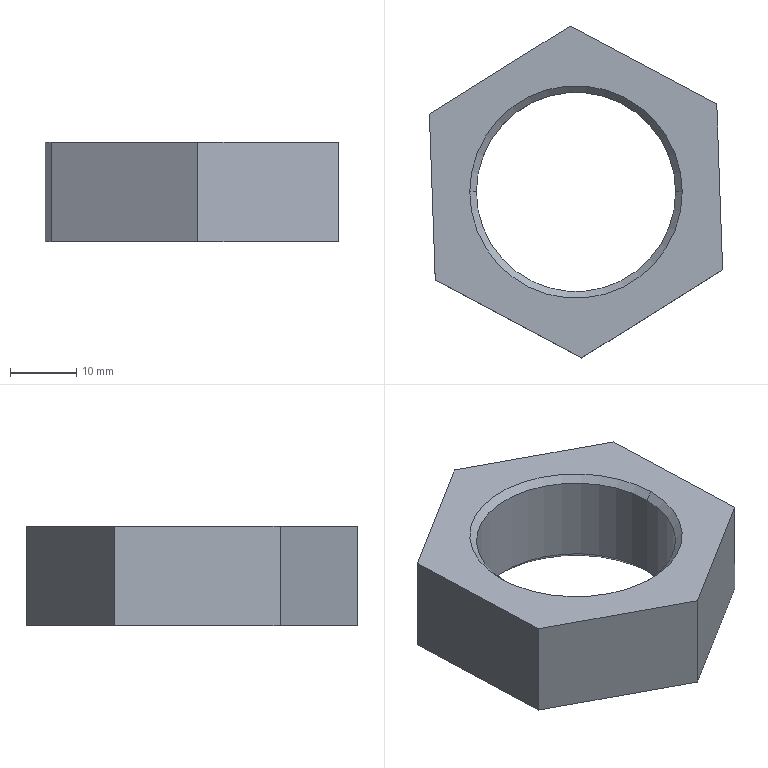Part | SolidWorks | features Chamfer 1, Extrusion 1 | 1 solid | 14 faces | box 44.157 x 49.969 x 15 mm | volume 13658 mm3 | plane 8 | cone 4 | cylinder 2 | commonest cylinder face diameters 30 x2
STEP:
#1=CARTESIAN_POINT('',(15.,0.,1.));
#2=VERTEX_POINT('',#1);
#3=CARTESIAN_POINT('',(-15.,0.,1.));
#4=VERTEX_POINT('',#3);
#5=CARTESIAN_POINT('',(0.,0.,1.));
#6=DIRECTION('',(0.,0.,-1.));
#7=DIRECTION('',(1.,0.,0.));
#8=AXIS2_PLACEMENT_3D('',#5,#6,#7);
#9=CIRCLE('',#8,15.);
#10=EDGE_CURVE('',#2,#4,#9,.T.);
#11=ORIENTED_EDGE('',*,*,#10,.F.);
#12=CARTESIAN_POINT('',(16.,0.,0.));
#13=VERTEX_POINT('',#12);
#14=CARTESIAN_POINT('',(16.,0.,0.));
#15=DIRECTION('',(0.7071,0.,-0.7071));
#16=VECTOR('',#15,1000.);
#17=LINE('',#14,#16);
#18=EDGE_CURVE('',#2,#13,#17,.T.);
#19=ORIENTED_EDGE('',*,*,#18,.T.);
#20=CARTESIAN_POINT('',(-16.,0.,0.));
#21=VERTEX_POINT('',#20);
#22=CARTESIAN_POINT('',(0.,0.,0.));
#23=DIRECTION('',(0.,0.,1.));
#24=DIRECTION('',(1.,0.,0.));
#25=AXIS2_PLACEMENT_3D('',#22,#23,#24);
#26=CIRCLE('',#25,16.);
#27=EDGE_CURVE('',#21,#13,#26,.T.);
#28=ORIENTED_EDGE('',*,*,#27,.F.);
#29=CARTESIAN_POINT('',(-16.,0.,0.));
#30=DIRECTION('',(-0.7071,0.,-0.7071));
#31=VECTOR('',#30,1000.);
#32=LINE('',#29,#31);
#33=EDGE_CURVE('',#4,#21,#32,.T.);
#34=ORIENTED_EDGE('',*,*,#33,.F.);
#35=EDGE_LOOP('',(#11,#19,#28,#34));
#36=FACE_OUTER_BOUND('',#35,.T.);
#37=CARTESIAN_POINT('',(0.,0.,0.));
#38=DIRECTION('',(0.,0.,-1.));
#39=DIRECTION('',(-1.,0.,0.));
#40=AXIS2_PLACEMENT_3D('',#37,#38,#39);
#41=CONICAL_SURFACE('',#40,16.,0.7854);
#42=ADVANCED_FACE('',(#36),#41,.F.);
#43=CARTESIAN_POINT('',(-15.,0.,14.));
#44=VERTEX_POINT('',#43);
#45=CARTESIAN_POINT('',(15.,0.,14.));
#46=VERTEX_POINT('',#45);
#47=CARTESIAN_POINT('',(0.,0.,14.));
#48=DIRECTION('',(0.,0.,1.));
#49=DIRECTION('',(1.,0.,0.));
#50=AXIS2_PLACEMENT_3D('',#47,#48,#49);
#51=CIRCLE('',#50,15.);
#52=EDGE_CURVE('',#44,#46,#51,.T.);
#53=ORIENTED_EDGE('',*,*,#52,.F.);
#54=CARTESIAN_POINT('',(-16.,0.,15.));
#55=VERTEX_POINT('',#54);
#56=CARTESIAN_POINT('',(-15.,0.,14.));
#57=DIRECTION('',(-0.7071,0.,0.7071));
#58=VECTOR('',#57,1000.);
#59=LINE('',#56,#58);
#60=EDGE_CURVE('',#44,#55,#59,.T.);
#61=ORIENTED_EDGE('',*,*,#60,.T.);
#62=CARTESIAN_POINT('',(16.,0.,15.));
#63=VERTEX_POINT('',#62);
#64=CARTESIAN_POINT('',(0.,0.,15.));
#65=DIRECTION('',(0.,0.,-1.));
#66=DIRECTION('',(1.,0.,0.));
#67=AXIS2_PLACEMENT_3D('',#64,#65,#66);
#68=CIRCLE('',#67,16.);
#69=EDGE_CURVE('',#63,#55,#68,.T.);
#70=ORIENTED_EDGE('',*,*,#69,.F.);
#71=CARTESIAN_POINT('',(15.,0.,14.));
#72=DIRECTION('',(0.7071,0.,0.7071));
#73=VECTOR('',#72,1000.);
#74=LINE('',#71,#73);
#75=EDGE_CURVE('',#46,#63,#74,.T.);
#76=ORIENTED_EDGE('',*,*,#75,.F.);
#77=EDGE_LOOP('',(#53,#61,#70,#76));
#78=FACE_OUTER_BOUND('',#77,.T.);
#79=CARTESIAN_POINT('',(0.,0.,14.));
#80=DIRECTION('',(0.,0.,1.));
#81=DIRECTION('',(1.,0.,0.));
#82=AXIS2_PLACEMENT_3D('',#79,#80,#81);
#83=CONICAL_SURFACE('',#82,15.,0.7854);
#84=ADVANCED_FACE('',(#78),#83,.F.);
#85=ORIENTED_EDGE('',*,*,#52,.T.);
#86=CARTESIAN_POINT('',(15.,0.,15.));
#87=DIRECTION('',(0.,0.,-1.));
#88=VECTOR('',#87,1000.);
#89=LINE('',#86,#88);
#90=EDGE_CURVE('',#46,#2,#89,.T.);
#91=ORIENTED_EDGE('',*,*,#90,.T.);
#92=ORIENTED_EDGE('',*,*,#10,.T.);
#93=CARTESIAN_POINT('',(-15.,0.,15.));
#94=DIRECTION('',(0.,0.,-1.));
#95=VECTOR('',#94,1000.);
#96=LINE('',#93,#95);
#97=EDGE_CURVE('',#44,#4,#96,.T.);
#98=ORIENTED_EDGE('',*,*,#97,.F.);
#99=EDGE_LOOP('',(#85,#91,#92,#98));
#100=FACE_OUTER_BOUND('',#99,.T.);
#101=CARTESIAN_POINT('',(0.,0.,15.));
#102=DIRECTION('',(0.,0.,-1.));
#103=DIRECTION('',(-1.,0.,0.));
#104=AXIS2_PLACEMENT_3D('',#101,#102,#103);
#105=CYLINDRICAL_SURFACE('',#104,15.);
#106=ADVANCED_FACE('',(#100),#105,.F.);
#107=ORIENTED_EDGE('',*,*,#69,.T.);
#108=CARTESIAN_POINT('',(0.,0.,15.));
#109=DIRECTION('',(0.,0.,-1.));
#110=DIRECTION('',(1.,0.,0.));
#111=AXIS2_PLACEMENT_3D('',#108,#109,#110);
#112=CIRCLE('',#111,16.);
#113=EDGE_CURVE('',#55,#63,#112,.T.);
#114=ORIENTED_EDGE('',*,*,#113,.T.);
#115=EDGE_LOOP('',(#107,#114));
#116=FACE_BOUND('',#115,.T.);
#117=CARTESIAN_POINT('',(0.8832,-24.984,15.));
#118=VERTEX_POINT('',#117);
#119=CARTESIAN_POINT('',(22.079,-11.727,15.));
#120=VERTEX_POINT('',#119);
#121=CARTESIAN_POINT('',(0.8832,-24.984,15.));
#122=DIRECTION('',(0.8478,0.5303,0.));
#123=VECTOR('',#122,1000.);
#124=LINE('',#121,#123);
#125=EDGE_CURVE('',#118,#120,#124,.T.);
#126=ORIENTED_EDGE('',*,*,#125,.T.);
#127=CARTESIAN_POINT('',(21.195,13.257,15.));
#128=VERTEX_POINT('',#127);
#129=CARTESIAN_POINT('',(22.079,-11.727,15.));
#130=DIRECTION('',(-0.03533,0.9994,0.));
#131=VECTOR('',#130,1000.);
#132=LINE('',#129,#131);
#133=EDGE_CURVE('',#120,#128,#132,.T.);
#134=ORIENTED_EDGE('',*,*,#133,.T.);
#135=CARTESIAN_POINT('',(-0.8832,24.984,15.));
#136=VERTEX_POINT('',#135);
#137=CARTESIAN_POINT('',(21.195,13.257,15.));
#138=DIRECTION('',(-0.8831,0.4691,0.));
#139=VECTOR('',#138,1000.);
#140=LINE('',#137,#139);
#141=EDGE_CURVE('',#128,#136,#140,.T.);
#142=ORIENTED_EDGE('',*,*,#141,.T.);
#143=CARTESIAN_POINT('',(-22.079,11.727,15.));
#144=VERTEX_POINT('',#143);
#145=CARTESIAN_POINT('',(-0.8832,24.984,15.));
#146=DIRECTION('',(-0.8478,-0.5303,0.));
#147=VECTOR('',#146,1000.);
#148=LINE('',#145,#147);
#149=EDGE_CURVE('',#136,#144,#148,.T.);
#150=ORIENTED_EDGE('',*,*,#149,.T.);
#151=CARTESIAN_POINT('',(-21.195,-13.257,15.));
#152=VERTEX_POINT('',#151);
#153=CARTESIAN_POINT('',(-22.079,11.727,15.));
#154=DIRECTION('',(0.03533,-0.9994,0.));
#155=VECTOR('',#154,1000.);
#156=LINE('',#153,#155);
#157=EDGE_CURVE('',#144,#152,#156,.T.);
#158=ORIENTED_EDGE('',*,*,#157,.T.);
#159=CARTESIAN_POINT('',(-21.195,-13.257,15.));
#160=DIRECTION('',(0.8831,-0.4691,0.));
#161=VECTOR('',#160,1000.);
#162=LINE('',#159,#161);
#163=EDGE_CURVE('',#152,#118,#162,.T.);
#164=ORIENTED_EDGE('',*,*,#163,.T.);
#165=EDGE_LOOP('',(#126,#134,#142,#150,#158,#164));
#166=FACE_OUTER_BOUND('',#165,.T.);
#167=CARTESIAN_POINT('',(0.,0.,15.));
#168=DIRECTION('',(0.,0.,1.));
#169=DIRECTION('',(1.,0.,0.));
#170=AXIS2_PLACEMENT_3D('',#167,#168,#169);
#171=PLANE('',#170);
#172=ADVANCED_FACE('',(#116,#166),#171,.T.);
#173=ORIENTED_EDGE('',*,*,#27,.T.);
#174=CARTESIAN_POINT('',(0.,0.,0.));
#175=DIRECTION('',(0.,0.,1.));
#176=DIRECTION('',(1.,0.,0.));
#177=AXIS2_PLACEMENT_3D('',#174,#175,#176);
#178=CIRCLE('',#177,16.);
#179=EDGE_CURVE('',#13,#21,#178,.T.);
#180=ORIENTED_EDGE('',*,*,#179,.T.);
#181=EDGE_LOOP('',(#173,#180));
#182=FACE_BOUND('',#181,.T.);
#183=CARTESIAN_POINT('',(0.8832,-24.984,0.));
#184=VERTEX_POINT('',#183);
#185=CARTESIAN_POINT('',(22.079,-11.727,0.));
#186=VERTEX_POINT('',#185);
#187=CARTESIAN_POINT('',(0.8832,-24.984,0.));
#188=DIRECTION('',(0.8478,0.5303,0.));
#189=VECTOR('',#188,1000.);
#190=LINE('',#187,#189);
#191=EDGE_CURVE('',#184,#186,#190,.T.);
#192=ORIENTED_EDGE('',*,*,#191,.F.);
#193=CARTESIAN_POINT('',(-21.195,-13.257,0.));
#194=VERTEX_POINT('',#193);
#195=CARTESIAN_POINT('',(-21.195,-13.257,0.));
#196=DIRECTION('',(0.8831,-0.4691,0.));
#197=VECTOR('',#196,1000.);
#198=LINE('',#195,#197);
#199=EDGE_CURVE('',#194,#184,#198,.T.);
#200=ORIENTED_EDGE('',*,*,#199,.F.);
#201=CARTESIAN_POINT('',(-22.079,11.727,0.));
#202=VERTEX_POINT('',#201);
#203=CARTESIAN_POINT('',(-22.079,11.727,0.));
#204=DIRECTION('',(0.03533,-0.9994,0.));
#205=VECTOR('',#204,1000.);
#206=LINE('',#203,#205);
#207=EDGE_CURVE('',#202,#194,#206,.T.);
#208=ORIENTED_EDGE('',*,*,#207,.F.);
#209=CARTESIAN_POINT('',(-0.8832,24.984,0.));
#210=VERTEX_POINT('',#209);
#211=CARTESIAN_POINT('',(-0.8832,24.984,0.));
#212=DIRECTION('',(-0.8478,-0.5303,0.));
#213=VECTOR('',#212,1000.);
#214=LINE('',#211,#213);
#215=EDGE_CURVE('',#210,#202,#214,.T.);
#216=ORIENTED_EDGE('',*,*,#215,.F.);
#217=CARTESIAN_POINT('',(21.195,13.257,0.));
#218=VERTEX_POINT('',#217);
#219=CARTESIAN_POINT('',(21.195,13.257,0.));
#220=DIRECTION('',(-0.8831,0.4691,0.));
#221=VECTOR('',#220,1000.);
#222=LINE('',#219,#221);
#223=EDGE_CURVE('',#218,#210,#222,.T.);
#224=ORIENTED_EDGE('',*,*,#223,.F.);
#225=CARTESIAN_POINT('',(22.079,-11.727,0.));
#226=DIRECTION('',(-0.03533,0.9994,0.));
#227=VECTOR('',#226,1000.);
#228=LINE('',#225,#227);
#229=EDGE_CURVE('',#186,#218,#228,.T.);
#230=ORIENTED_EDGE('',*,*,#229,.F.);
#231=EDGE_LOOP('',(#192,#200,#208,#216,#224,#230));
#232=FACE_OUTER_BOUND('',#231,.T.);
#233=CARTESIAN_POINT('',(0.,0.,0.));
#234=DIRECTION('',(0.,0.,1.));
#235=DIRECTION('',(1.,0.,0.));
#236=AXIS2_PLACEMENT_3D('',#233,#234,#235);
#237=PLANE('',#236);
#238=ADVANCED_FACE('',(#182,#232),#237,.F.);
#239=ORIENTED_EDGE('',*,*,#191,.T.);
#240=CARTESIAN_POINT('',(22.079,-11.727,15.));
#241=DIRECTION('',(0.,0.,-1.));
#242=VECTOR('',#241,1000.);
#243=LINE('',#240,#242);
#244=EDGE_CURVE('',#120,#186,#243,.T.);
#245=ORIENTED_EDGE('',*,*,#244,.F.);
#246=ORIENTED_EDGE('',*,*,#125,.F.);
#247=CARTESIAN_POINT('',(0.8832,-24.984,15.));
#248=DIRECTION('',(0.,0.,-1.));
#249=VECTOR('',#248,1000.);
#250=LINE('',#247,#249);
#251=EDGE_CURVE('',#118,#184,#250,.T.);
#252=ORIENTED_EDGE('',*,*,#251,.T.);
#253=EDGE_LOOP('',(#239,#245,#246,#252));
#254=FACE_OUTER_BOUND('',#253,.T.);
#255=CARTESIAN_POINT('',(0.8832,-24.984,15.));
#256=DIRECTION('',(-0.5303,0.8478,0.));
#257=DIRECTION('',(-0.8478,-0.5303,0.));
#258=AXIS2_PLACEMENT_3D('',#255,#256,#257);
#259=PLANE('',#258);
#260=ADVANCED_FACE('',(#254),#259,.F.);
#261=ORIENTED_EDGE('',*,*,#229,.T.);
#262=CARTESIAN_POINT('',(21.195,13.257,15.));
#263=DIRECTION('',(0.,0.,-1.));
#264=VECTOR('',#263,1000.);
#265=LINE('',#262,#264);
#266=EDGE_CURVE('',#128,#218,#265,.T.);
#267=ORIENTED_EDGE('',*,*,#266,.F.);
#268=ORIENTED_EDGE('',*,*,#133,.F.);
#269=ORIENTED_EDGE('',*,*,#244,.T.);
#270=EDGE_LOOP('',(#261,#267,#268,#269));
#271=FACE_OUTER_BOUND('',#270,.T.);
#272=CARTESIAN_POINT('',(22.079,-11.727,15.));
#273=DIRECTION('',(-0.9994,-0.03533,0.));
#274=DIRECTION('',(0.03533,-0.9994,0.));
#275=AXIS2_PLACEMENT_3D('',#272,#273,#274);
#276=PLANE('',#275);
#277=ADVANCED_FACE('',(#271),#276,.F.);
#278=ORIENTED_EDGE('',*,*,#223,.T.);
#279=CARTESIAN_POINT('',(-0.8832,24.984,15.));
#280=DIRECTION('',(0.,0.,-1.));
#281=VECTOR('',#280,1000.);
#282=LINE('',#279,#281);
#283=EDGE_CURVE('',#136,#210,#282,.T.);
#284=ORIENTED_EDGE('',*,*,#283,.F.);
#285=ORIENTED_EDGE('',*,*,#141,.F.);
#286=ORIENTED_EDGE('',*,*,#266,.T.);
#287=EDGE_LOOP('',(#278,#284,#285,#286));
#288=FACE_OUTER_BOUND('',#287,.T.);
#289=CARTESIAN_POINT('',(21.195,13.257,15.));
#290=DIRECTION('',(-0.4691,-0.8831,0.));
#291=DIRECTION('',(0.8831,-0.4691,0.));
#292=AXIS2_PLACEMENT_3D('',#289,#290,#291);
#293=PLANE('',#292);
#294=ADVANCED_FACE('',(#288),#293,.F.);
#295=ORIENTED_EDGE('',*,*,#215,.T.);
#296=CARTESIAN_POINT('',(-22.079,11.727,15.));
#297=DIRECTION('',(0.,0.,-1.));
#298=VECTOR('',#297,1000.);
#299=LINE('',#296,#298);
#300=EDGE_CURVE('',#144,#202,#299,.T.);
#301=ORIENTED_EDGE('',*,*,#300,.F.);
#302=ORIENTED_EDGE('',*,*,#149,.F.);
#303=ORIENTED_EDGE('',*,*,#283,.T.);
#304=EDGE_LOOP('',(#295,#301,#302,#303));
#305=FACE_OUTER_BOUND('',#304,.T.);
#306=CARTESIAN_POINT('',(-0.8832,24.984,15.));
#307=DIRECTION('',(0.5303,-0.8478,0.));
#308=DIRECTION('',(0.8478,0.5303,0.));
#309=AXIS2_PLACEMENT_3D('',#306,#307,#308);
#310=PLANE('',#309);
#311=ADVANCED_FACE('',(#305),#310,.F.);
#312=ORIENTED_EDGE('',*,*,#207,.T.);
#313=CARTESIAN_POINT('',(-21.195,-13.257,15.));
#314=DIRECTION('',(0.,0.,-1.));
#315=VECTOR('',#314,1000.);
#316=LINE('',#313,#315);
#317=EDGE_CURVE('',#152,#194,#316,.T.);
#318=ORIENTED_EDGE('',*,*,#317,.F.);
#319=ORIENTED_EDGE('',*,*,#157,.F.);
#320=ORIENTED_EDGE('',*,*,#300,.T.);
#321=EDGE_LOOP('',(#312,#318,#319,#320));
#322=FACE_OUTER_BOUND('',#321,.T.);
#323=CARTESIAN_POINT('',(-22.079,11.727,15.));
#324=DIRECTION('',(0.9994,0.03533,0.));
#325=DIRECTION('',(-0.03533,0.9994,0.));
#326=AXIS2_PLACEMENT_3D('',#323,#324,#325);
#327=PLANE('',#326);
#328=ADVANCED_FACE('',(#322),#327,.F.);
#329=ORIENTED_EDGE('',*,*,#199,.T.);
#330=ORIENTED_EDGE('',*,*,#251,.F.);
#331=ORIENTED_EDGE('',*,*,#163,.F.);
#332=ORIENTED_EDGE('',*,*,#317,.T.);
#333=EDGE_LOOP('',(#329,#330,#331,#332));
#334=FACE_OUTER_BOUND('',#333,.T.);
#335=CARTESIAN_POINT('',(-21.195,-13.257,15.));
#336=DIRECTION('',(0.4691,0.8831,0.));
#337=DIRECTION('',(-0.8831,0.4691,0.));
#338=AXIS2_PLACEMENT_3D('',#335,#336,#337);
#339=PLANE('',#338);
#340=ADVANCED_FACE('',(#334),#339,.F.);
#341=ORIENTED_EDGE('',*,*,#90,.F.);
#342=CARTESIAN_POINT('',(0.,0.,14.));
#343=DIRECTION('',(0.,0.,1.));
#344=DIRECTION('',(1.,0.,0.));
#345=AXIS2_PLACEMENT_3D('',#342,#343,#344);
#346=CIRCLE('',#345,15.);
#347=EDGE_CURVE('',#46,#44,#346,.T.);
#348=ORIENTED_EDGE('',*,*,#347,.T.);
#349=ORIENTED_EDGE('',*,*,#97,.T.);
#350=CARTESIAN_POINT('',(0.,0.,1.));
#351=DIRECTION('',(0.,0.,-1.));
#352=DIRECTION('',(1.,0.,0.));
#353=AXIS2_PLACEMENT_3D('',#350,#351,#352);
#354=CIRCLE('',#353,15.);
#355=EDGE_CURVE('',#4,#2,#354,.T.);
#356=ORIENTED_EDGE('',*,*,#355,.T.);
#357=EDGE_LOOP('',(#341,#348,#349,#356));
#358=FACE_OUTER_BOUND('',#357,.T.);
#359=CARTESIAN_POINT('',(0.,0.,15.));
#360=DIRECTION('',(0.,0.,-1.));
#361=DIRECTION('',(-1.,0.,0.));
#362=AXIS2_PLACEMENT_3D('',#359,#360,#361);
#363=CYLINDRICAL_SURFACE('',#362,15.);
#364=ADVANCED_FACE('',(#358),#363,.F.);
#365=ORIENTED_EDGE('',*,*,#60,.F.);
#366=ORIENTED_EDGE('',*,*,#347,.F.);
#367=ORIENTED_EDGE('',*,*,#75,.T.);
#368=ORIENTED_EDGE('',*,*,#113,.F.);
#369=EDGE_LOOP('',(#365,#366,#367,#368));
#370=FACE_OUTER_BOUND('',#369,.T.);
#371=CARTESIAN_POINT('',(0.,0.,14.));
#372=DIRECTION('',(0.,0.,1.));
#373=DIRECTION('',(1.,0.,0.));
#374=AXIS2_PLACEMENT_3D('',#371,#372,#373);
#375=CONICAL_SURFACE('',#374,15.,0.7854);
#376=ADVANCED_FACE('',(#370),#375,.F.);
#377=ORIENTED_EDGE('',*,*,#18,.F.);
#378=ORIENTED_EDGE('',*,*,#355,.F.);
#379=ORIENTED_EDGE('',*,*,#33,.T.);
#380=ORIENTED_EDGE('',*,*,#179,.F.);
#381=EDGE_LOOP('',(#377,#378,#379,#380));
#382=FACE_OUTER_BOUND('',#381,.T.);
#383=CARTESIAN_POINT('',(0.,0.,0.));
#384=DIRECTION('',(0.,0.,-1.));
#385=DIRECTION('',(-1.,0.,0.));
#386=AXIS2_PLACEMENT_3D('',#383,#384,#385);
#387=CONICAL_SURFACE('',#386,16.,0.7854);
#388=ADVANCED_FACE('',(#382),#387,.F.);
#389=CLOSED_SHELL('',(#42,#84,#106,#172,#238,#260,#277,#294,#311,#328,#340,#364,#376,#388));
#390=MANIFOLD_SOLID_BREP('',#389);
#391=CARTESIAN_POINT('',(0.,0.,0.));
#392=DIRECTION('',(0.,0.,1.));
#393=DIRECTION('',(1.,0.,0.));
#394=AXIS2_PLACEMENT_3D('',#391,#392,#393);
#395=(LENGTH_UNIT()NAMED_UNIT(*)SI_UNIT(.MILLI.,.METRE.));
#396=UNCERTAINTY_MEASURE_WITH_UNIT(LENGTH_MEASURE(0.00001),#395,'','');
#397=(NAMED_UNIT(*)PLANE_ANGLE_UNIT()SI_UNIT($,.RADIAN.));
#398=(NAMED_UNIT(*)SI_UNIT($,.STERADIAN.)SOLID_ANGLE_UNIT());
#399=(GEOMETRIC_REPRESENTATION_CONTEXT(3)GLOBAL_UNCERTAINTY_ASSIGNED_CONTEXT((#396))GLOBAL_UNIT_ASSIGNED_CONTEXT((#395,#397,#398))REPRESENTATION_CONTEXT('',''));
#400=ADVANCED_BREP_SHAPE_REPRESENTATION('',(#390,#394),#399);